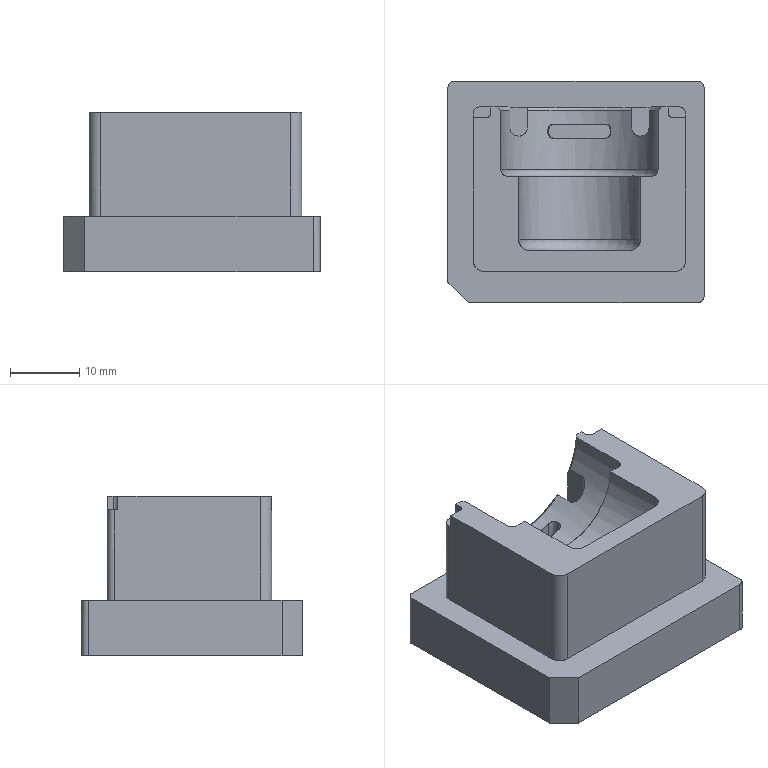CAM job | PowerMill | 3-axis milling, other | part box 37 x 32 x 23 mm
Tools:
number,name,type,diameter,tip_radius,length,cutting_length,overhang,flutes,holder,toolpaths_using
1,D10C,end_mill,10.0,0.0,60.0,,30.0,1,D42L35,2
15,D3C,end_mill,3.0,0.0,30.0,,15.0,1,D42L35,2
1,D10C_1_1_1,end_mill,10.0,0.0,60.0,,23.44,1,D42L35,3
15,D3C_1_1,end_mill,3.0,0.0,30.0,,11.32,1,D42L35,2
26,D1.5C_1_1,end_mill,1.5,0.0,6.56,,13.34,1,D42L35,1
3,D10_1_1_1,end_mill,10.0,0.0,60.0,,23.16,1,D42L35,8
22,R1.5_1_1,ball_nosed,3.0,1.5,30.0,,12.4,1,D42L35,1
6,R0.5_1_1,ball_nosed,1.0,0.5,8.2,,11.36,1,D42L35,1
20,D1.5_1_1,end_mill,1.5,0.0,6.72,,13.46,1,D42L35,2
8,D1_1_1,end_mill,1.0,0.0,3.0,,2.32,1,D42L35,2
13,Text_D4_1_1,taper_spherical,4.0,0.3,60.0,,15.28,1,D42L35,2
1,D10C_2_1_1,end_mill,10.0,0.0,60.0,,23.44,1,D42L35,3
26,D1.5C_2_1,end_mill,1.5,0.0,6.68,,13.34,1,D42L35,1
22,R1.5_2_1,ball_nosed,3.0,1.5,30.0,,12.36,1,D42L35,1
6,R0.5_2_1,ball_nosed,1.0,0.5,6.84,,11.36,1,D42L35,1
20,D1.5_2_1,end_mill,1.5,0.0,6.84,,13.42,1,D42L35,2
Operations:
program,toolpath,strategy,tool,tool_number,tool_diameter,tip_radius,flutes,spindle_rpm,feed_cut,surface_speed_m_min_computed,feed_per_tooth_computed,tolerance,thickness,stepover,stepdown,cut_length,cut_time_min,total_time_min,workplane
06-C01-6-F,精公开粗01-扫面平行-D10C,raster_area_clear,D10C_1_1_1,1,10.0,0.0,1.0,8000.0,10000.0,251.33,1.25,0.03,0.28,6.0,1.0,378.04,0.038,0.0442,
06-C01-6-F,精公开粗01-外形偏置-D10C,offset_area_clear,D10C_1_1_1,1,10.0,0.0,1.0,8000.0,10000.0,251.33,1.25,0.03,0.28,6.0,1.0,12838.268,1.284,1.379,
06-C01-6-F,精公开粗01-基准台等高-D10C,constantz,D10C_1_1_1,1,10.0,0.0,1.0,8000.0,10000.0,251.33,1.25,0.03,0.07,5.0,0.4,3669.043,0.367,0.3781,
06-C01-6-F,精公再粗02-外形偏置-D3C,offset_area_clear,D3C_1_1,15,3.0,0.0,1.0,18000.0,5000.0,169.65,0.2778,0.03,0.0,2.0,1.0,11607.582,2.321,2.435,
06-C01-6-F,精公再粗03-外形偏置-D1.5C,offset_area_clear,D1.5C_1_1,26,1.5,0.0,1.0,20000.0,3000.0,94.25,0.15,0.03,0.0,0.7,1.0,2559.843,0.853,1.417,
06-C01-6-F,精公基准台01-平坦面平行-D10,raster_area_clear,D10_1_1_1,3,10.0,0.0,1.0,8500.0,600.0,267.04,0.0706,0.005,0.38,5.0,1.0,283.347,0.472,0.5369,
06-C01-6-F,精公基准台01-基准面偏置-D10,offset_area_clear,D10_1_1_1,3,10.0,0.0,1.0,8500.0,600.0,267.04,0.0706,0.005,0.38,5.0,1.0,149.1,0.248,0.2683,
06-C01-6-F,精公基准台01-外形侧光-D10,profile_area_clear,D10_1_1_1,3,10.0,0.0,1.0,8500.0,600.0,267.04,0.0706,0.005,-0.07,0.08,1.0,275.852,0.46,0.482,
06-C01-6-F,精公基准台01-基准台侧光-D10,profile_area_clear,D10_1_1_1,3,10.0,0.0,1.0,8500.0,600.0,267.04,0.0706,0.005,0.0,0.08,1.0,333.234,0.555,0.6215,
06-C01-6-F,精公精光01-最佳等高-R1.5,opti_constz,R1.5_1_1,22,3.0,1.5,1.0,22000.0,2000.0,207.35,0.0909,0.005,-0.075,0.04,1.0,15793.784,7.897,8.467,
06-C01-6-F,精公精光02-清角-R0.5,automatic_corner,R0.5_1_1,6,1.0,0.5,1.0,20000.0,1000.0,62.83,0.05,0.005,-0.075,5.0,1.0,6289.106,6.289,6.668,
06-C01-6-F,精公精光03-等高-D1.5,constantz,D1.5_1_1,20,1.5,0.0,1.0,20000.0,1500.0,94.25,0.075,0.005,-0.075,5.0,0.03,4469.827,2.98,3.283,
06-C01-6-F,精公精光03-平坦面偏置-D1.5,offset_area_clear,D1.5_1_1,20,1.5,0.0,1.0,20000.0,600.0,94.25,0.03,0.005,0.0,0.7,1.0,50.31,0.084,0.1889,
06-C01-6-F,精公精光04-等高-D1,constantz,D1_1_1,8,1.0,0.0,1.0,20000.0,1000.0,62.83,0.05,0.005,-0.075,5.0,0.02,734.373,0.734,0.8485,
06-C01-6-F,精公刻字01-刻字-Text_D4,pattern,Text_D4_1_1,13,4.0,0.3,1.0,15000.0,1000.0,188.5,0.0667,0.005,0.0,5.0,1.0,43.002,0.043,0.0699,
06-C01-6-R,粗公开粗01-扫面平行-D10C,raster_area_clear,D10C_2_1_1,1,10.0,0.0,1.0,8000.0,10000.0,251.33,1.25,0.03,0.15,6.0,1.0,375.7,0.038,0.0439,
06-C01-6-R,粗公开粗01-外形偏置-D10C,offset_area_clear,D10C_2_1_1,1,10.0,0.0,1.0,8000.0,10000.0,251.33,1.25,0.03,0.15,6.0,1.0,12780.295,1.278,1.374,
06-C01-6-R,粗公开粗01-基准台等高-D10C,constantz,D10C_2_1_1,1,10.0,0.0,1.0,8000.0,10000.0,251.33,1.25,0.03,0.07,5.0,0.4,3669.043,0.367,0.3781,
06-C01-6-R,粗公再粗02-外形偏置-D3C,offset_area_clear,D3C_1_1,15,3.0,0.0,1.0,18000.0,5000.0,169.65,0.2778,0.03,-0.13,2.0,1.0,11587.721,2.318,2.348,
06-C01-6-R,粗公再粗03-外形偏置-D1.5C,offset_area_clear,D1.5C_2_1,26,1.5,0.0,1.0,20000.0,3000.0,94.25,0.15,0.03,-0.13,0.7,1.0,2484.057,0.828,1.374,
06-C01-6-R,粗公基准台01-平坦面平行-D10,raster_area_clear,D10_1_1_1,3,10.0,0.0,1.0,8500.0,600.0,267.04,0.0706,0.01,0.25,5.0,1.0,270.622,0.451,0.532,
06-C01-6-R,粗公基准台01-基准面偏置-D10,offset_area_clear,D10_1_1_1,3,10.0,0.0,1.0,8500.0,600.0,267.04,0.0706,0.01,0.25,5.0,1.0,149.963,0.25,0.2697,
06-C01-6-R,粗公基准台01-外形侧光-D10,profile_area_clear,D10_1_1_1,3,10.0,0.0,1.0,8500.0,600.0,267.04,0.0706,0.01,-0.2,0.08,1.0,274.21,0.457,0.4792,
06-C01-6-R,粗公基准台01-基准台侧光-D10,profile_area_clear,D10_1_1_1,3,10.0,0.0,1.0,8500.0,600.0,267.04,0.0706,0.01,0.0,0.08,1.0,333.217,0.555,0.621,
06-C01-6-R,粗公精光01-最佳等高-R1.5,opti_constz,R1.5_2_1,22,3.0,1.5,1.0,22000.0,2000.0,207.35,0.0909,0.01,-0.205,0.048,1.0,13340.767,6.67,7.162,
06-C01-6-R,粗公精光02-清角-R0.5,automatic_corner,R0.5_2_1,6,1.0,0.5,1.0,20000.0,1000.0,62.83,0.05,0.01,-0.205,5.0,1.0,3106.57,3.107,3.28,
06-C01-6-R,粗公精光03-等高-D1.5,constantz,D1.5_2_1,20,1.5,0.0,1.0,20000.0,1500.0,94.25,0.075,0.01,-0.205,5.0,0.036,4227.51,2.818,3.13,
06-C01-6-R,粗公精光03-平坦面偏置-D1.5,offset_area_clear,D1.5_2_1,20,1.5,0.0,1.0,20000.0,600.0,94.25,0.03,0.01,-0.13,0.7,1.0,50.939,0.085,0.1898,
06-C01-6-R,粗公精光04-等高-D1,constantz,D1_1_1,8,1.0,0.0,1.0,20000.0,1000.0,62.83,0.05,0.01,-0.205,5.0,0.024,697.483,0.698,0.7945,
06-C01-6-R,粗公刻字01-刻字-Text_D4,pattern,Text_D4_1_1,13,4.0,0.3,1.0,15000.0,1000.0,188.5,0.0667,0.01,0.0,5.0,1.0,39.798,0.04,0.0653,
,精公开粗01-外形偏置-D10C_Reference,offset_area_clear,D10C,1,10.0,0.0,1.0,8000.0,10000.0,251.33,1.25,0.03,0.28,6.0,1.0,33814.292,3.381,3.627,
,精公再粗02-外形偏置-D3C_Reference,offset_area_clear,D3C,15,3.0,0.0,1.0,18000.0,5000.0,169.65,0.2778,0.03,0.0,2.0,1.0,43973.592,8.795,9.271,
,粗公开粗01-外形偏置-D10C_Reference,offset_area_clear,D10C,1,10.0,0.0,1.0,8000.0,10000.0,251.33,1.25,0.03,0.15,6.0,1.0,33320.088,3.332,3.576,
,粗公再粗02-外形偏置-D3C_Reference,offset_area_clear,D3C,15,3.0,0.0,1.0,18000.0,5000.0,169.65,0.2778,0.03,-0.13,2.0,1.0,43247.356,8.649,8.751,